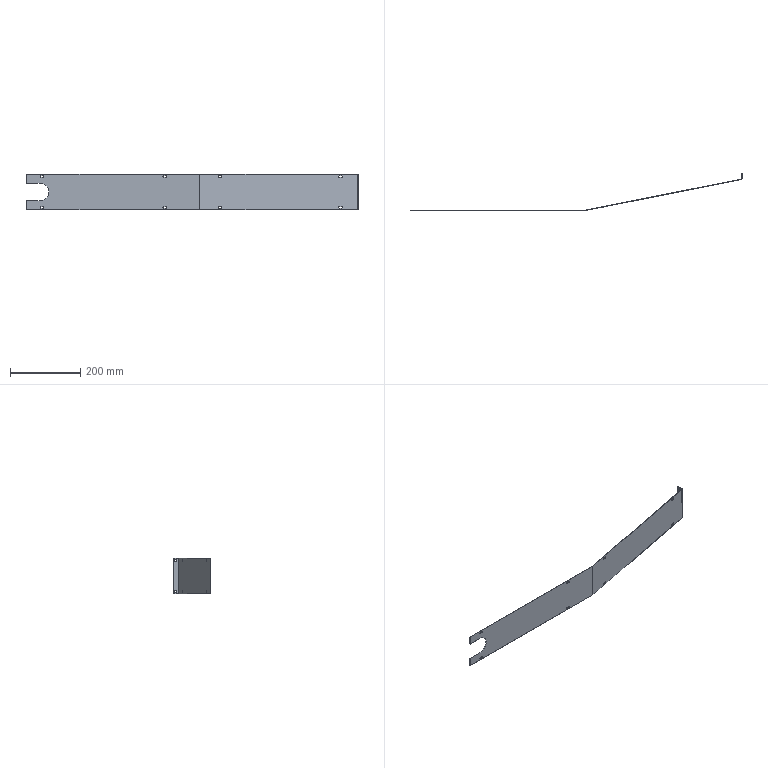Part | SolidWorks | features ICE 4, ExtruThin 1, Fillet 1 | 1 solid | 64 faces | box 946 x 108 x 100 mm | volume 93762 mm3 | cylinder 35 | plane 29 | commonest cylinder face diameters 5 x20 4 x10 7 x4 50 x1